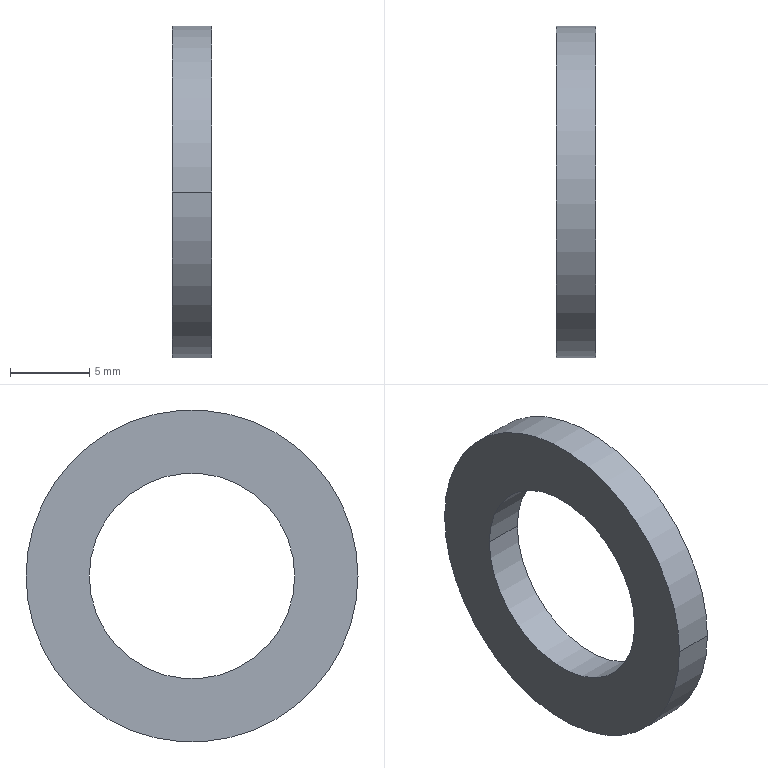Part | STEP file | KS B 1326 - 12x21 | 1 solid | 6 faces | box 2.5 x 21 x 21 mm | volume 534.071 mm3 | cylinder 4 | plane 2 | commonest cylinder face diameters 13 x2 21 x2
STEP:
#1=CARTESIAN_POINT('',(0.,0.,0.));
#2=DIRECTION('',(0.,0.,1.));
#3=DIRECTION('',(1.,0.,0.));
#4=AXIS2_PLACEMENT_3D('',#1,#2,#3);
#5=CARTESIAN_POINT('',(0.,-6.5,0.));
#6=VERTEX_POINT('',#5);
#7=CARTESIAN_POINT('',(2.5,-6.5,0.));
#8=VERTEX_POINT('',#7);
#9=CARTESIAN_POINT('',(0.,-6.5,0.));
#10=DIRECTION('',(1.,0.,0.));
#11=VECTOR('',#10,1.);
#12=LINE('',#9,#11);
#13=CARTESIAN_POINT('',(0.,0.,0.));
#14=DIRECTION('',(1.,0.,0.));
#15=DIRECTION('',(0.,-1.,0.));
#16=AXIS2_PLACEMENT_3D('',#13,#14,#15);
#17=CYLINDRICAL_SURFACE('',#16,6.5);
#18=CARTESIAN_POINT('',(6.283,0.));
#19=DIRECTION('',(0.,1.));
#20=VECTOR('',#19,1.);
#21=LINE('',#18,#20);
#22=(GEOMETRIC_REPRESENTATION_CONTEXT(2)PARAMETRIC_REPRESENTATION_CONTEXT()REPRESENTATION_CONTEXT('',''));
#23=DEFINITIONAL_REPRESENTATION('',(#21),#22);
#24=PCURVE('',#17,#23);
#25=CARTESIAN_POINT('',(0.,0.,0.));
#26=DIRECTION('',(1.,0.,0.));
#27=DIRECTION('',(0.,-1.,0.));
#28=AXIS2_PLACEMENT_3D('',#25,#26,#27);
#29=CYLINDRICAL_SURFACE('',#28,6.5);
#30=CARTESIAN_POINT('',(0.,0.));
#31=DIRECTION('',(0.,1.));
#32=VECTOR('',#31,1.);
#33=LINE('',#30,#32);
#34=(GEOMETRIC_REPRESENTATION_CONTEXT(2)PARAMETRIC_REPRESENTATION_CONTEXT()REPRESENTATION_CONTEXT('',''));
#35=DEFINITIONAL_REPRESENTATION('',(#33),#34);
#36=PCURVE('',#29,#35);
#37=SURFACE_CURVE('',#12,(#24,#36),.PCURVE_S1.);
#38=EDGE_CURVE('',#6,#8,#37,.T.);
#39=ORIENTED_EDGE('',*,*,#38,.T.);
#40=CARTESIAN_POINT('',(2.5,6.5,0.));
#41=VERTEX_POINT('',#40);
#42=CARTESIAN_POINT('',(2.5,0.,0.));
#43=DIRECTION('',(-1.,0.,0.));
#44=DIRECTION('',(0.,-1.,0.));
#45=AXIS2_PLACEMENT_3D('',#42,#43,#44);
#46=CIRCLE('',#45,6.5);
#47=CARTESIAN_POINT('',(6.283,2.5));
#48=DIRECTION('',(-1.,0.));
#49=VECTOR('',#48,1.);
#50=LINE('',#47,#49);
#51=(GEOMETRIC_REPRESENTATION_CONTEXT(2)PARAMETRIC_REPRESENTATION_CONTEXT()REPRESENTATION_CONTEXT('',''));
#52=DEFINITIONAL_REPRESENTATION('',(#50),#51);
#53=PCURVE('',#17,#52);
#54=CARTESIAN_POINT('',(2.5,0.,0.));
#55=DIRECTION('',(-1.,0.,0.));
#56=DIRECTION('',(0.,0.,1.));
#57=AXIS2_PLACEMENT_3D('',#54,#55,#56);
#58=PLANE('',#57);
#59=CARTESIAN_POINT('',(0.,0.));
#60=DIRECTION('',(0.,-1.));
#61=AXIS2_PLACEMENT_2D('',#59,#60);
#62=CIRCLE('',#61,6.5);
#63=(GEOMETRIC_REPRESENTATION_CONTEXT(2)PARAMETRIC_REPRESENTATION_CONTEXT()REPRESENTATION_CONTEXT('',''));
#64=DEFINITIONAL_REPRESENTATION('',(#62),#63);
#65=PCURVE('',#58,#64);
#66=SURFACE_CURVE('',#46,(#53,#65),.PCURVE_S1.);
#67=EDGE_CURVE('',#8,#41,#66,.T.);
#68=ORIENTED_EDGE('',*,*,#67,.T.);
#69=CARTESIAN_POINT('',(0.,6.5,0.));
#70=VERTEX_POINT('',#69);
#71=CARTESIAN_POINT('',(0.,6.5,0.));
#72=DIRECTION('',(1.,0.,0.));
#73=VECTOR('',#72,1.);
#74=LINE('',#71,#73);
#75=CARTESIAN_POINT('',(3.142,0.));
#76=DIRECTION('',(0.,1.));
#77=VECTOR('',#76,1.);
#78=LINE('',#75,#77);
#79=(GEOMETRIC_REPRESENTATION_CONTEXT(2)PARAMETRIC_REPRESENTATION_CONTEXT()REPRESENTATION_CONTEXT('',''));
#80=DEFINITIONAL_REPRESENTATION('',(#78),#79);
#81=PCURVE('',#17,#80);
#82=CARTESIAN_POINT('',(3.142,0.));
#83=DIRECTION('',(0.,1.));
#84=VECTOR('',#83,1.);
#85=LINE('',#82,#84);
#86=(GEOMETRIC_REPRESENTATION_CONTEXT(2)PARAMETRIC_REPRESENTATION_CONTEXT()REPRESENTATION_CONTEXT('',''));
#87=DEFINITIONAL_REPRESENTATION('',(#85),#86);
#88=PCURVE('',#29,#87);
#89=SURFACE_CURVE('',#74,(#81,#88),.PCURVE_S1.);
#90=EDGE_CURVE('',#70,#41,#89,.T.);
#91=ORIENTED_EDGE('',*,*,#90,.F.);
#92=CARTESIAN_POINT('',(0.,0.,0.));
#93=DIRECTION('',(1.,0.,0.));
#94=DIRECTION('',(0.,-1.,0.));
#95=AXIS2_PLACEMENT_3D('',#92,#93,#94);
#96=CIRCLE('',#95,6.5);
#97=CARTESIAN_POINT('',(0.,0.));
#98=DIRECTION('',(1.,0.));
#99=VECTOR('',#98,1.);
#100=LINE('',#97,#99);
#101=(GEOMETRIC_REPRESENTATION_CONTEXT(2)PARAMETRIC_REPRESENTATION_CONTEXT()REPRESENTATION_CONTEXT('',''));
#102=DEFINITIONAL_REPRESENTATION('',(#100),#101);
#103=PCURVE('',#17,#102);
#104=CARTESIAN_POINT('',(0.,0.,0.));
#105=DIRECTION('',(-1.,0.,0.));
#106=DIRECTION('',(0.,0.,1.));
#107=AXIS2_PLACEMENT_3D('',#104,#105,#106);
#108=PLANE('',#107);
#109=CARTESIAN_POINT('',(0.,-6.5));
#110=CARTESIAN_POINT('',(-11.258,-6.5));
#111=CARTESIAN_POINT('',(-5.629,3.25));
#112=CARTESIAN_POINT('',(0.,13.));
#113=CARTESIAN_POINT('',(5.629,3.25));
#114=CARTESIAN_POINT('',(11.258,-6.5));
#115=CARTESIAN_POINT('',(0.,-6.5));
#116=(BOUNDED_CURVE()B_SPLINE_CURVE(2,(#109,#110,#111,#112,#113,#114,#115),.UNSPECIFIED.,.T.,.F.)B_SPLINE_CURVE_WITH_KNOTS((1,2,2,2,2,1),(-2.094,0.,2.094,4.189,6.283,8.378),.UNSPECIFIED.)CURVE()GEOMETRIC_REPRESENTATION_ITEM()RATIONAL_B_SPLINE_CURVE((1.,0.5,1.,0.5,1.,0.5,1.))REPRESENTATION_ITEM(''));
#117=(GEOMETRIC_REPRESENTATION_CONTEXT(2)PARAMETRIC_REPRESENTATION_CONTEXT()REPRESENTATION_CONTEXT('',''));
#118=DEFINITIONAL_REPRESENTATION('',(#116),#117);
#119=PCURVE('',#108,#118);
#120=SURFACE_CURVE('',#96,(#103,#119),.PCURVE_S1.);
#121=EDGE_CURVE('',#70,#6,#120,.T.);
#122=ORIENTED_EDGE('',*,*,#121,.T.);
#123=EDGE_LOOP('',(#39,#68,#91,#122));
#124=FACE_BOUND('',#123,.F.);
#125=ADVANCED_FACE('',(#124),#17,.F.);
#126=CARTESIAN_POINT('',(0.,10.5,0.));
#127=VERTEX_POINT('',#126);
#128=CARTESIAN_POINT('',(0.,-10.5,0.));
#129=VERTEX_POINT('',#128);
#130=CARTESIAN_POINT('',(0.,0.,0.));
#131=DIRECTION('',(-1.,0.,0.));
#132=DIRECTION('',(0.,-1.,0.));
#133=AXIS2_PLACEMENT_3D('',#130,#131,#132);
#134=CIRCLE('',#133,10.5);
#135=CARTESIAN_POINT('',(0.,0.,0.));
#136=DIRECTION('',(1.,0.,0.));
#137=DIRECTION('',(0.,-1.,0.));
#138=AXIS2_PLACEMENT_3D('',#135,#136,#137);
#139=CYLINDRICAL_SURFACE('',#138,10.5);
#140=CARTESIAN_POINT('',(6.283,0.));
#141=DIRECTION('',(-1.,0.));
#142=VECTOR('',#141,1.);
#143=LINE('',#140,#142);
#144=(GEOMETRIC_REPRESENTATION_CONTEXT(2)PARAMETRIC_REPRESENTATION_CONTEXT()REPRESENTATION_CONTEXT('',''));
#145=DEFINITIONAL_REPRESENTATION('',(#143),#144);
#146=PCURVE('',#139,#145);
#147=CARTESIAN_POINT('',(0.,0.));
#148=DIRECTION('',(0.,-1.));
#149=AXIS2_PLACEMENT_2D('',#147,#148);
#150=CIRCLE('',#149,10.5);
#151=(GEOMETRIC_REPRESENTATION_CONTEXT(2)PARAMETRIC_REPRESENTATION_CONTEXT()REPRESENTATION_CONTEXT('',''));
#152=DEFINITIONAL_REPRESENTATION('',(#150),#151);
#153=PCURVE('',#108,#152);
#154=SURFACE_CURVE('',#134,(#146,#153),.PCURVE_S1.);
#155=EDGE_CURVE('',#127,#129,#154,.T.);
#156=ORIENTED_EDGE('',*,*,#155,.F.);
#157=CARTESIAN_POINT('',(2.5,10.5,0.));
#158=VERTEX_POINT('',#157);
#159=CARTESIAN_POINT('',(0.,10.5,0.));
#160=DIRECTION('',(1.,0.,0.));
#161=VECTOR('',#160,1.);
#162=LINE('',#159,#161);
#163=CARTESIAN_POINT('',(3.142,0.));
#164=DIRECTION('',(0.,1.));
#165=VECTOR('',#164,1.);
#166=LINE('',#163,#165);
#167=(GEOMETRIC_REPRESENTATION_CONTEXT(2)PARAMETRIC_REPRESENTATION_CONTEXT()REPRESENTATION_CONTEXT('',''));
#168=DEFINITIONAL_REPRESENTATION('',(#166),#167);
#169=PCURVE('',#139,#168);
#170=CARTESIAN_POINT('',(0.,0.,0.));
#171=DIRECTION('',(1.,0.,0.));
#172=DIRECTION('',(0.,-1.,0.));
#173=AXIS2_PLACEMENT_3D('',#170,#171,#172);
#174=CYLINDRICAL_SURFACE('',#173,10.5);
#175=CARTESIAN_POINT('',(3.142,0.));
#176=DIRECTION('',(0.,1.));
#177=VECTOR('',#176,1.);
#178=LINE('',#175,#177);
#179=(GEOMETRIC_REPRESENTATION_CONTEXT(2)PARAMETRIC_REPRESENTATION_CONTEXT()REPRESENTATION_CONTEXT('',''));
#180=DEFINITIONAL_REPRESENTATION('',(#178),#179);
#181=PCURVE('',#174,#180);
#182=SURFACE_CURVE('',#162,(#169,#181),.PCURVE_S1.);
#183=EDGE_CURVE('',#127,#158,#182,.T.);
#184=ORIENTED_EDGE('',*,*,#183,.T.);
#185=CARTESIAN_POINT('',(2.5,-10.5,0.));
#186=VERTEX_POINT('',#185);
#187=CARTESIAN_POINT('',(2.5,0.,0.));
#188=DIRECTION('',(-1.,0.,0.));
#189=DIRECTION('',(0.,-1.,0.));
#190=AXIS2_PLACEMENT_3D('',#187,#188,#189);
#191=CIRCLE('',#190,10.5);
#192=CARTESIAN_POINT('',(6.283,2.5));
#193=DIRECTION('',(-1.,0.));
#194=VECTOR('',#193,1.);
#195=LINE('',#192,#194);
#196=(GEOMETRIC_REPRESENTATION_CONTEXT(2)PARAMETRIC_REPRESENTATION_CONTEXT()REPRESENTATION_CONTEXT('',''));
#197=DEFINITIONAL_REPRESENTATION('',(#195),#196);
#198=PCURVE('',#139,#197);
#199=CARTESIAN_POINT('',(0.,0.));
#200=DIRECTION('',(0.,-1.));
#201=AXIS2_PLACEMENT_2D('',#199,#200);
#202=CIRCLE('',#201,10.5);
#203=(GEOMETRIC_REPRESENTATION_CONTEXT(2)PARAMETRIC_REPRESENTATION_CONTEXT()REPRESENTATION_CONTEXT('',''));
#204=DEFINITIONAL_REPRESENTATION('',(#202),#203);
#205=PCURVE('',#58,#204);
#206=SURFACE_CURVE('',#191,(#198,#205),.PCURVE_S1.);
#207=EDGE_CURVE('',#158,#186,#206,.T.);
#208=ORIENTED_EDGE('',*,*,#207,.T.);
#209=CARTESIAN_POINT('',(0.,-10.5,0.));
#210=DIRECTION('',(1.,0.,0.));
#211=VECTOR('',#210,1.);
#212=LINE('',#209,#211);
#213=CARTESIAN_POINT('',(0.,0.));
#214=DIRECTION('',(0.,1.));
#215=VECTOR('',#214,1.);
#216=LINE('',#213,#215);
#217=(GEOMETRIC_REPRESENTATION_CONTEXT(2)PARAMETRIC_REPRESENTATION_CONTEXT()REPRESENTATION_CONTEXT('',''));
#218=DEFINITIONAL_REPRESENTATION('',(#216),#217);
#219=PCURVE('',#139,#218);
#220=CARTESIAN_POINT('',(6.283,0.));
#221=DIRECTION('',(0.,1.));
#222=VECTOR('',#221,1.);
#223=LINE('',#220,#222);
#224=(GEOMETRIC_REPRESENTATION_CONTEXT(2)PARAMETRIC_REPRESENTATION_CONTEXT()REPRESENTATION_CONTEXT('',''));
#225=DEFINITIONAL_REPRESENTATION('',(#223),#224);
#226=PCURVE('',#174,#225);
#227=SURFACE_CURVE('',#212,(#219,#226),.PCURVE_S1.);
#228=EDGE_CURVE('',#129,#186,#227,.T.);
#229=ORIENTED_EDGE('',*,*,#228,.F.);
#230=EDGE_LOOP('',(#156,#184,#208,#229));
#231=FACE_BOUND('',#230,.T.);
#232=ADVANCED_FACE('',(#231),#139,.T.);
#233=CARTESIAN_POINT('',(0.,0.,0.));
#234=DIRECTION('',(1.,0.,0.));
#235=DIRECTION('',(0.,-1.,0.));
#236=AXIS2_PLACEMENT_3D('',#233,#234,#235);
#237=CIRCLE('',#236,6.5);
#238=CARTESIAN_POINT('',(0.,-6.5));
#239=CARTESIAN_POINT('',(-11.258,-6.5));
#240=CARTESIAN_POINT('',(-5.629,3.25));
#241=CARTESIAN_POINT('',(0.,13.));
#242=CARTESIAN_POINT('',(5.629,3.25));
#243=CARTESIAN_POINT('',(11.258,-6.5));
#244=CARTESIAN_POINT('',(0.,-6.5));
#245=(BOUNDED_CURVE()B_SPLINE_CURVE(2,(#238,#239,#240,#241,#242,#243,#244),.UNSPECIFIED.,.T.,.F.)B_SPLINE_CURVE_WITH_KNOTS((1,2,2,2,2,1),(-2.094,0.,2.094,4.189,6.283,8.378),.UNSPECIFIED.)CURVE()GEOMETRIC_REPRESENTATION_ITEM()RATIONAL_B_SPLINE_CURVE((1.,0.5,1.,0.5,1.,0.5,1.))REPRESENTATION_ITEM(''));
#246=(GEOMETRIC_REPRESENTATION_CONTEXT(2)PARAMETRIC_REPRESENTATION_CONTEXT()REPRESENTATION_CONTEXT('',''));
#247=DEFINITIONAL_REPRESENTATION('',(#245),#246);
#248=PCURVE('',#108,#247);
#249=CARTESIAN_POINT('',(0.,0.));
#250=DIRECTION('',(1.,0.));
#251=VECTOR('',#250,1.);
#252=LINE('',#249,#251);
#253=(GEOMETRIC_REPRESENTATION_CONTEXT(2)PARAMETRIC_REPRESENTATION_CONTEXT()REPRESENTATION_CONTEXT('',''));
#254=DEFINITIONAL_REPRESENTATION('',(#252),#253);
#255=PCURVE('',#29,#254);
#256=SURFACE_CURVE('',#237,(#248,#255),.PCURVE_S1.);
#257=EDGE_CURVE('',#6,#70,#256,.T.);
#258=ORIENTED_EDGE('',*,*,#257,.T.);
#259=ORIENTED_EDGE('',*,*,#121,.T.);
#260=EDGE_LOOP('',(#258,#259));
#261=FACE_BOUND('',#260,.T.);
#262=CARTESIAN_POINT('',(0.,0.,0.));
#263=DIRECTION('',(-1.,0.,0.));
#264=DIRECTION('',(0.,-1.,0.));
#265=AXIS2_PLACEMENT_3D('',#262,#263,#264);
#266=CIRCLE('',#265,10.5);
#267=CARTESIAN_POINT('',(0.,0.));
#268=DIRECTION('',(0.,-1.));
#269=AXIS2_PLACEMENT_2D('',#267,#268);
#270=CIRCLE('',#269,10.5);
#271=(GEOMETRIC_REPRESENTATION_CONTEXT(2)PARAMETRIC_REPRESENTATION_CONTEXT()REPRESENTATION_CONTEXT('',''));
#272=DEFINITIONAL_REPRESENTATION('',(#270),#271);
#273=PCURVE('',#108,#272);
#274=CARTESIAN_POINT('',(6.283,0.));
#275=DIRECTION('',(-1.,0.));
#276=VECTOR('',#275,1.);
#277=LINE('',#274,#276);
#278=(GEOMETRIC_REPRESENTATION_CONTEXT(2)PARAMETRIC_REPRESENTATION_CONTEXT()REPRESENTATION_CONTEXT('',''));
#279=DEFINITIONAL_REPRESENTATION('',(#277),#278);
#280=PCURVE('',#174,#279);
#281=SURFACE_CURVE('',#266,(#273,#280),.PCURVE_S1.);
#282=EDGE_CURVE('',#129,#127,#281,.T.);
#283=ORIENTED_EDGE('',*,*,#282,.T.);
#284=ORIENTED_EDGE('',*,*,#155,.T.);
#285=EDGE_LOOP('',(#283,#284));
#286=FACE_BOUND('',#285,.T.);
#287=ADVANCED_FACE('',(#261,#286),#108,.T.);
#288=ORIENTED_EDGE('',*,*,#67,.T.);
#289=CARTESIAN_POINT('',(2.5,0.,0.));
#290=DIRECTION('',(-1.,0.,0.));
#291=DIRECTION('',(0.,-1.,0.));
#292=AXIS2_PLACEMENT_3D('',#289,#290,#291);
#293=CIRCLE('',#292,6.5);
#294=CARTESIAN_POINT('',(0.,0.));
#295=DIRECTION('',(0.,-1.));
#296=AXIS2_PLACEMENT_2D('',#294,#295);
#297=CIRCLE('',#296,6.5);
#298=(GEOMETRIC_REPRESENTATION_CONTEXT(2)PARAMETRIC_REPRESENTATION_CONTEXT()REPRESENTATION_CONTEXT('',''));
#299=DEFINITIONAL_REPRESENTATION('',(#297),#298);
#300=PCURVE('',#58,#299);
#301=CARTESIAN_POINT('',(6.283,2.5));
#302=DIRECTION('',(-1.,0.));
#303=VECTOR('',#302,1.);
#304=LINE('',#301,#303);
#305=(GEOMETRIC_REPRESENTATION_CONTEXT(2)PARAMETRIC_REPRESENTATION_CONTEXT()REPRESENTATION_CONTEXT('',''));
#306=DEFINITIONAL_REPRESENTATION('',(#304),#305);
#307=PCURVE('',#29,#306);
#308=SURFACE_CURVE('',#293,(#300,#307),.PCURVE_S1.);
#309=EDGE_CURVE('',#41,#8,#308,.T.);
#310=ORIENTED_EDGE('',*,*,#309,.T.);
#311=EDGE_LOOP('',(#288,#310));
#312=FACE_BOUND('',#311,.T.);
#313=CARTESIAN_POINT('',(2.5,0.,0.));
#314=DIRECTION('',(-1.,0.,0.));
#315=DIRECTION('',(0.,-1.,0.));
#316=AXIS2_PLACEMENT_3D('',#313,#314,#315);
#317=CIRCLE('',#316,10.5);
#318=CARTESIAN_POINT('',(0.,0.));
#319=DIRECTION('',(0.,-1.));
#320=AXIS2_PLACEMENT_2D('',#318,#319);
#321=CIRCLE('',#320,10.5);
#322=(GEOMETRIC_REPRESENTATION_CONTEXT(2)PARAMETRIC_REPRESENTATION_CONTEXT()REPRESENTATION_CONTEXT('',''));
#323=DEFINITIONAL_REPRESENTATION('',(#321),#322);
#324=PCURVE('',#58,#323);
#325=CARTESIAN_POINT('',(6.283,2.5));
#326=DIRECTION('',(-1.,0.));
#327=VECTOR('',#326,1.);
#328=LINE('',#325,#327);
#329=(GEOMETRIC_REPRESENTATION_CONTEXT(2)PARAMETRIC_REPRESENTATION_CONTEXT()REPRESENTATION_CONTEXT('',''));
#330=DEFINITIONAL_REPRESENTATION('',(#328),#329);
#331=PCURVE('',#174,#330);
#332=SURFACE_CURVE('',#317,(#324,#331),.PCURVE_S1.);
#333=EDGE_CURVE('',#186,#158,#332,.T.);
#334=ORIENTED_EDGE('',*,*,#333,.F.);
#335=ORIENTED_EDGE('',*,*,#207,.F.);
#336=EDGE_LOOP('',(#334,#335));
#337=FACE_BOUND('',#336,.T.);
#338=ADVANCED_FACE('',(#312,#337),#58,.F.);
#339=ORIENTED_EDGE('',*,*,#183,.F.);
#340=ORIENTED_EDGE('',*,*,#282,.F.);
#341=ORIENTED_EDGE('',*,*,#228,.T.);
#342=ORIENTED_EDGE('',*,*,#333,.T.);
#343=EDGE_LOOP('',(#339,#340,#341,#342));
#344=FACE_BOUND('',#343,.T.);
#345=ADVANCED_FACE('',(#344),#174,.T.);
#346=ORIENTED_EDGE('',*,*,#309,.T.);
#347=ORIENTED_EDGE('',*,*,#38,.F.);
#348=ORIENTED_EDGE('',*,*,#257,.T.);
#349=ORIENTED_EDGE('',*,*,#90,.T.);
#350=EDGE_LOOP('',(#346,#347,#348,#349));
#351=FACE_BOUND('',#350,.F.);
#352=ADVANCED_FACE('',(#351),#29,.F.);
#353=CLOSED_SHELL('',(#125,#232,#287,#338,#345,#352));
#354=MANIFOLD_SOLID_BREP('',#353);
#355=(LENGTH_UNIT()NAMED_UNIT(*)SI_UNIT(.MILLI.,.METRE.));
#356=UNCERTAINTY_MEASURE_WITH_UNIT(LENGTH_MEASURE(0.0000001),#355,'','');
#357=(NAMED_UNIT(*)PLANE_ANGLE_UNIT()SI_UNIT($,.RADIAN.));
#358=(NAMED_UNIT(*)SI_UNIT($,.STERADIAN.)SOLID_ANGLE_UNIT());
#359=(GEOMETRIC_REPRESENTATION_CONTEXT(3)GLOBAL_UNCERTAINTY_ASSIGNED_CONTEXT((#356))GLOBAL_UNIT_ASSIGNED_CONTEXT((#355,#357,#358))REPRESENTATION_CONTEXT('',''));
#360=ADVANCED_BREP_SHAPE_REPRESENTATION('',(#4,#354),#359);